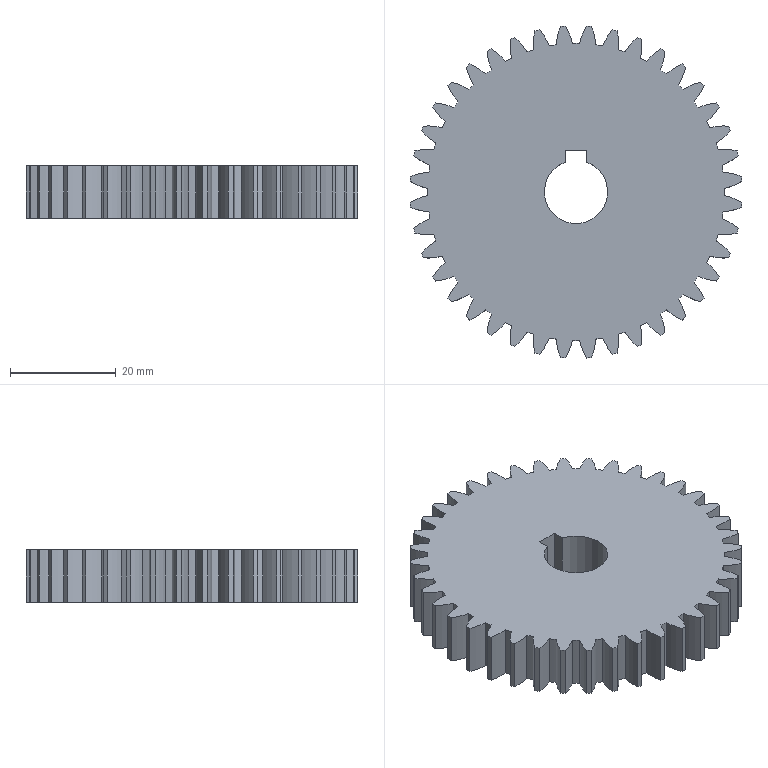Part | NX | features BREP 1 | 1 solid | 166 faces | box 62.872 x 62.872 x 10 mm | volume 26610 mm3 | cylinder 161 | plane 5 | commonest cylinder face diameters 24 x80 56.248 x40 63 x40 12 x1